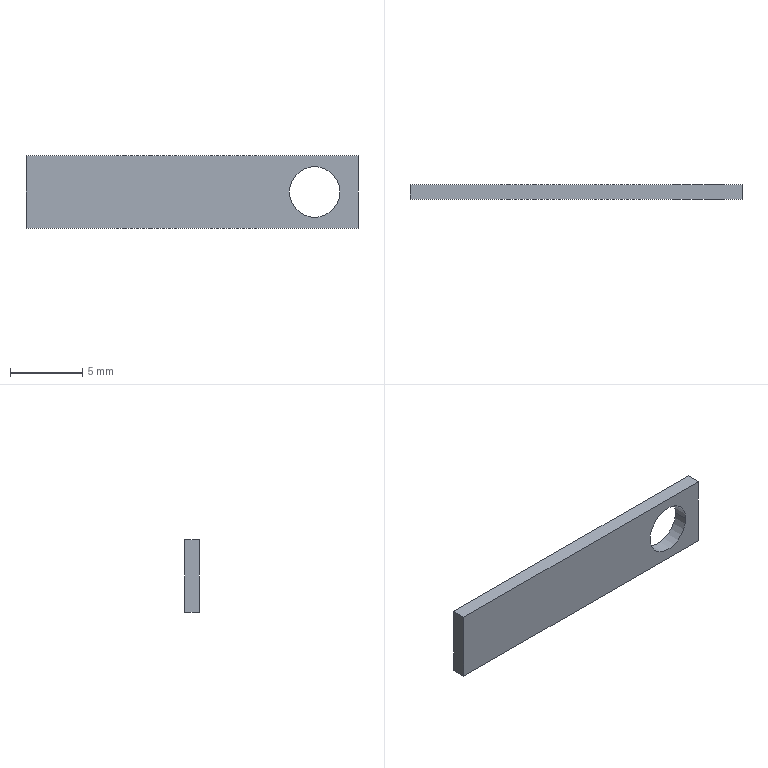Part | NX | 1 solid | 8 faces | box 23 x 1 x 5 mm | volume 105.379 mm3 | plane 6 | cylinder 2 | commonest cylinder face diameters 3.5 x2
STEP:
#1=CARTESIAN_POINT('',(-11.5,-0.5,0.));
#2=VERTEX_POINT('',#1);
#3=CARTESIAN_POINT('',(-11.5,0.5,0.));
#4=VERTEX_POINT('',#3);
#5=CARTESIAN_POINT('',(-11.5,-0.5,0.));
#6=DIRECTION('',(0.,1.,0.));
#7=VECTOR('',#6,1000.);
#8=LINE('',#5,#7);
#9=EDGE_CURVE('',#2,#4,#8,.T.);
#10=ORIENTED_EDGE('',*,*,#9,.T.);
#11=CARTESIAN_POINT('',(11.5,0.5,0.));
#12=VERTEX_POINT('',#11);
#13=CARTESIAN_POINT('',(-11.5,0.5,0.));
#14=DIRECTION('',(1.,0.,0.));
#15=VECTOR('',#14,1000.);
#16=LINE('',#13,#15);
#17=EDGE_CURVE('',#4,#12,#16,.T.);
#18=ORIENTED_EDGE('',*,*,#17,.T.);
#19=CARTESIAN_POINT('',(11.5,-0.5,0.));
#20=VERTEX_POINT('',#19);
#21=CARTESIAN_POINT('',(11.5,0.5,0.));
#22=DIRECTION('',(0.,-1.,0.));
#23=VECTOR('',#22,1000.);
#24=LINE('',#21,#23);
#25=EDGE_CURVE('',#12,#20,#24,.T.);
#26=ORIENTED_EDGE('',*,*,#25,.T.);
#27=CARTESIAN_POINT('',(11.5,-0.5,0.));
#28=DIRECTION('',(-1.,0.,0.));
#29=VECTOR('',#28,1000.);
#30=LINE('',#27,#29);
#31=EDGE_CURVE('',#20,#2,#30,.T.);
#32=ORIENTED_EDGE('',*,*,#31,.T.);
#33=EDGE_LOOP('',(#10,#18,#26,#32));
#34=FACE_BOUND('',#33,.T.);
#35=CARTESIAN_POINT('',(0.,0.,0.));
#36=DIRECTION('',(0.,0.,1.));
#37=DIRECTION('',(1.,0.,0.));
#38=AXIS2_PLACEMENT_3D('',#35,#36,#37);
#39=PLANE('',#38);
#40=ADVANCED_FACE('',(#34),#39,.F.);
#41=ORIENTED_EDGE('',*,*,#9,.F.);
#42=CARTESIAN_POINT('',(-11.5,-0.5,5.));
#43=VERTEX_POINT('',#42);
#44=CARTESIAN_POINT('',(-11.5,-0.5,5.));
#45=DIRECTION('',(0.,0.,-1.));
#46=VECTOR('',#45,1000.);
#47=LINE('',#44,#46);
#48=EDGE_CURVE('',#43,#2,#47,.T.);
#49=ORIENTED_EDGE('',*,*,#48,.F.);
#50=CARTESIAN_POINT('',(-11.5,0.5,5.));
#51=VERTEX_POINT('',#50);
#52=CARTESIAN_POINT('',(-11.5,-0.5,5.));
#53=DIRECTION('',(0.,1.,0.));
#54=VECTOR('',#53,1000.);
#55=LINE('',#52,#54);
#56=EDGE_CURVE('',#43,#51,#55,.T.);
#57=ORIENTED_EDGE('',*,*,#56,.T.);
#58=CARTESIAN_POINT('',(-11.5,0.5,5.));
#59=DIRECTION('',(0.,0.,-1.));
#60=VECTOR('',#59,1000.);
#61=LINE('',#58,#60);
#62=EDGE_CURVE('',#51,#4,#61,.T.);
#63=ORIENTED_EDGE('',*,*,#62,.T.);
#64=EDGE_LOOP('',(#41,#49,#57,#63));
#65=FACE_BOUND('',#64,.T.);
#66=CARTESIAN_POINT('',(-11.5,0.5,0.));
#67=DIRECTION('',(-1.,0.,0.));
#68=DIRECTION('',(0.,0.,1.));
#69=AXIS2_PLACEMENT_3D('',#66,#67,#68);
#70=PLANE('',#69);
#71=ADVANCED_FACE('',(#65),#70,.T.);
#72=ORIENTED_EDGE('',*,*,#17,.F.);
#73=ORIENTED_EDGE('',*,*,#62,.F.);
#74=CARTESIAN_POINT('',(11.5,0.5,5.));
#75=VERTEX_POINT('',#74);
#76=CARTESIAN_POINT('',(-11.5,0.5,5.));
#77=DIRECTION('',(1.,0.,0.));
#78=VECTOR('',#77,1000.);
#79=LINE('',#76,#78);
#80=EDGE_CURVE('',#51,#75,#79,.T.);
#81=ORIENTED_EDGE('',*,*,#80,.T.);
#82=CARTESIAN_POINT('',(11.5,0.5,5.));
#83=DIRECTION('',(0.,0.,-1.));
#84=VECTOR('',#83,1000.);
#85=LINE('',#82,#84);
#86=EDGE_CURVE('',#75,#12,#85,.T.);
#87=ORIENTED_EDGE('',*,*,#86,.T.);
#88=EDGE_LOOP('',(#72,#73,#81,#87));
#89=FACE_BOUND('',#88,.T.);
#90=CARTESIAN_POINT('',(10.25,0.5,2.5));
#91=VERTEX_POINT('',#90);
#92=CARTESIAN_POINT('',(6.75,0.5,2.5));
#93=VERTEX_POINT('',#92);
#94=CARTESIAN_POINT('',(8.5,0.5,2.5));
#95=DIRECTION('',(0.,1.,0.));
#96=DIRECTION('',(1.,0.,0.));
#97=AXIS2_PLACEMENT_3D('',#94,#95,#96);
#98=CIRCLE('',#97,1.75);
#99=EDGE_CURVE('',#91,#93,#98,.T.);
#100=ORIENTED_EDGE('',*,*,#99,.F.);
#101=CARTESIAN_POINT('',(8.5,0.5,2.5));
#102=DIRECTION('',(0.,1.,0.));
#103=DIRECTION('',(1.,0.,0.));
#104=AXIS2_PLACEMENT_3D('',#101,#102,#103);
#105=CIRCLE('',#104,1.75);
#106=EDGE_CURVE('',#93,#91,#105,.T.);
#107=ORIENTED_EDGE('',*,*,#106,.F.);
#108=EDGE_LOOP('',(#100,#107));
#109=FACE_BOUND('',#108,.T.);
#110=CARTESIAN_POINT('',(11.5,0.5,0.));
#111=DIRECTION('',(0.,1.,0.));
#112=DIRECTION('',(1.,0.,0.));
#113=AXIS2_PLACEMENT_3D('',#110,#111,#112);
#114=PLANE('',#113);
#115=ADVANCED_FACE('',(#89,#109),#114,.T.);
#116=ORIENTED_EDGE('',*,*,#25,.F.);
#117=ORIENTED_EDGE('',*,*,#86,.F.);
#118=CARTESIAN_POINT('',(11.5,-0.5,5.));
#119=VERTEX_POINT('',#118);
#120=CARTESIAN_POINT('',(11.5,0.5,5.));
#121=DIRECTION('',(0.,-1.,0.));
#122=VECTOR('',#121,1000.);
#123=LINE('',#120,#122);
#124=EDGE_CURVE('',#75,#119,#123,.T.);
#125=ORIENTED_EDGE('',*,*,#124,.T.);
#126=CARTESIAN_POINT('',(11.5,-0.5,5.));
#127=DIRECTION('',(0.,0.,-1.));
#128=VECTOR('',#127,1000.);
#129=LINE('',#126,#128);
#130=EDGE_CURVE('',#119,#20,#129,.T.);
#131=ORIENTED_EDGE('',*,*,#130,.T.);
#132=EDGE_LOOP('',(#116,#117,#125,#131));
#133=FACE_BOUND('',#132,.T.);
#134=CARTESIAN_POINT('',(11.5,-0.5,0.));
#135=DIRECTION('',(1.,0.,0.));
#136=DIRECTION('',(0.,1.,0.));
#137=AXIS2_PLACEMENT_3D('',#134,#135,#136);
#138=PLANE('',#137);
#139=ADVANCED_FACE('',(#133),#138,.T.);
#140=ORIENTED_EDGE('',*,*,#31,.F.);
#141=ORIENTED_EDGE('',*,*,#130,.F.);
#142=CARTESIAN_POINT('',(11.5,-0.5,5.));
#143=DIRECTION('',(-1.,0.,0.));
#144=VECTOR('',#143,1000.);
#145=LINE('',#142,#144);
#146=EDGE_CURVE('',#119,#43,#145,.T.);
#147=ORIENTED_EDGE('',*,*,#146,.T.);
#148=ORIENTED_EDGE('',*,*,#48,.T.);
#149=EDGE_LOOP('',(#140,#141,#147,#148));
#150=FACE_BOUND('',#149,.T.);
#151=CARTESIAN_POINT('',(10.25,-0.5,2.5));
#152=VERTEX_POINT('',#151);
#153=CARTESIAN_POINT('',(6.75,-0.5,2.5));
#154=VERTEX_POINT('',#153);
#155=CARTESIAN_POINT('',(8.5,-0.5,2.5));
#156=DIRECTION('',(0.,-1.,0.));
#157=DIRECTION('',(-1.,0.,0.));
#158=AXIS2_PLACEMENT_3D('',#155,#156,#157);
#159=CIRCLE('',#158,1.75);
#160=EDGE_CURVE('',#152,#154,#159,.T.);
#161=ORIENTED_EDGE('',*,*,#160,.F.);
#162=CARTESIAN_POINT('',(8.5,-0.5,2.5));
#163=DIRECTION('',(0.,-1.,0.));
#164=DIRECTION('',(-1.,0.,0.));
#165=AXIS2_PLACEMENT_3D('',#162,#163,#164);
#166=CIRCLE('',#165,1.75);
#167=EDGE_CURVE('',#154,#152,#166,.T.);
#168=ORIENTED_EDGE('',*,*,#167,.F.);
#169=EDGE_LOOP('',(#161,#168));
#170=FACE_BOUND('',#169,.T.);
#171=CARTESIAN_POINT('',(-11.5,-0.5,0.));
#172=DIRECTION('',(0.,-1.,0.));
#173=DIRECTION('',(0.,0.,-1.));
#174=AXIS2_PLACEMENT_3D('',#171,#172,#173);
#175=PLANE('',#174);
#176=ADVANCED_FACE('',(#150,#170),#175,.T.);
#177=ORIENTED_EDGE('',*,*,#56,.F.);
#178=ORIENTED_EDGE('',*,*,#146,.F.);
#179=ORIENTED_EDGE('',*,*,#124,.F.);
#180=ORIENTED_EDGE('',*,*,#80,.F.);
#181=EDGE_LOOP('',(#177,#178,#179,#180));
#182=FACE_BOUND('',#181,.T.);
#183=CARTESIAN_POINT('',(0.,0.,5.));
#184=DIRECTION('',(0.,0.,1.));
#185=DIRECTION('',(1.,0.,0.));
#186=AXIS2_PLACEMENT_3D('',#183,#184,#185);
#187=PLANE('',#186);
#188=ADVANCED_FACE('',(#182),#187,.T.);
#189=ORIENTED_EDGE('',*,*,#99,.T.);
#190=CARTESIAN_POINT('',(6.75,0.5,2.5));
#191=DIRECTION('',(0.,-1.,0.));
#192=VECTOR('',#191,1000.);
#193=LINE('',#190,#192);
#194=EDGE_CURVE('',#154,#93,#193,.F.);
#195=ORIENTED_EDGE('',*,*,#194,.F.);
#196=ORIENTED_EDGE('',*,*,#167,.T.);
#197=CARTESIAN_POINT('',(10.25,0.5,2.5));
#198=DIRECTION('',(0.,-1.,0.));
#199=VECTOR('',#198,1000.);
#200=LINE('',#197,#199);
#201=EDGE_CURVE('',#152,#91,#200,.F.);
#202=ORIENTED_EDGE('',*,*,#201,.T.);
#203=EDGE_LOOP('',(#189,#195,#196,#202));
#204=FACE_BOUND('',#203,.T.);
#205=CARTESIAN_POINT('',(8.5,0.5,2.5));
#206=DIRECTION('',(0.,-1.,0.));
#207=DIRECTION('',(1.,0.,0.));
#208=AXIS2_PLACEMENT_3D('',#205,#206,#207);
#209=CYLINDRICAL_SURFACE('',#208,1.75);
#210=ADVANCED_FACE('',(#204),#209,.F.);
#211=ORIENTED_EDGE('',*,*,#160,.T.);
#212=ORIENTED_EDGE('',*,*,#194,.T.);
#213=ORIENTED_EDGE('',*,*,#106,.T.);
#214=ORIENTED_EDGE('',*,*,#201,.F.);
#215=EDGE_LOOP('',(#211,#212,#213,#214));
#216=FACE_BOUND('',#215,.T.);
#217=CARTESIAN_POINT('',(8.5,0.5,2.5));
#218=DIRECTION('',(0.,-1.,0.));
#219=DIRECTION('',(1.,0.,0.));
#220=AXIS2_PLACEMENT_3D('',#217,#218,#219);
#221=CYLINDRICAL_SURFACE('',#220,1.75);
#222=ADVANCED_FACE('',(#216),#221,.F.);
#223=CLOSED_SHELL('',(#40,#71,#115,#139,#176,#188,#210,#222));
#224=MANIFOLD_SOLID_BREP('',#223);
#225=(LENGTH_UNIT()NAMED_UNIT(*)SI_UNIT(.MILLI.,.METRE.));
#226=UNCERTAINTY_MEASURE_WITH_UNIT(LENGTH_MEASURE(0.00001),#225,'','');
#227=(NAMED_UNIT(*)PLANE_ANGLE_UNIT()SI_UNIT($,.RADIAN.));
#228=(NAMED_UNIT(*)SI_UNIT($,.STERADIAN.)SOLID_ANGLE_UNIT());
#229=(GEOMETRIC_REPRESENTATION_CONTEXT(3)GLOBAL_UNCERTAINTY_ASSIGNED_CONTEXT((#226))GLOBAL_UNIT_ASSIGNED_CONTEXT((#225,#227,#228))REPRESENTATION_CONTEXT('',''));
#230=ADVANCED_BREP_SHAPE_REPRESENTATION('',(#224),#229);